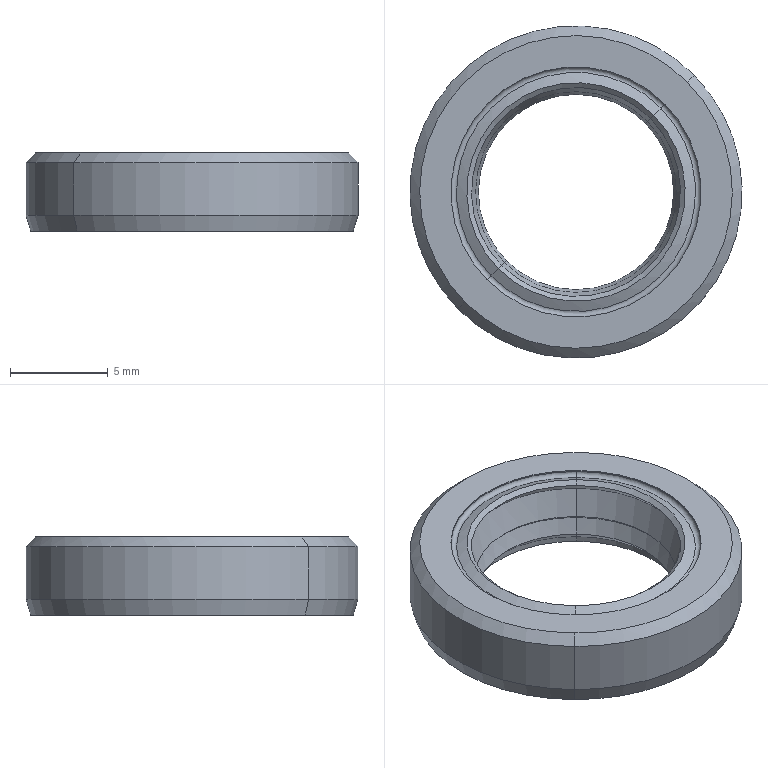Part | SolidWorks | features BaseBody 1 | 1 solid | 53 faces | box 17 x 17 x 4 mm | volume 314.365 mm3 | cone 22 | cylinder 14 | torus 10 | plane 7 | commonest cylinder face diameters 11 x2 12.8 x2 13.5 x2 13.6 x2 15.2 x2 16.2 x2
STEP:
#1=CARTESIAN_POINT('',(387.744,107.08,47.545));
#2=VERTEX_POINT('',#1);
#3=CARTESIAN_POINT('',(387.336,106.678,46.9));
#4=VERTEX_POINT('',#3);
#5=CARTESIAN_POINT('',(387.799,107.135,46.9));
#6=DIRECTION('',(0.7022,-0.712,0.));
#7=DIRECTION('',(0.712,0.7022,0.));
#8=AXIS2_PLACEMENT_3D('',#5,#6,#7);
#9=CIRCLE('',#8,0.65);
#10=EDGE_CURVE('',#2,#4,#9,.T.);
#11=ORIENTED_EDGE('',*,*,#10,.T.);
#12=CARTESIAN_POINT('',(378.864,98.322,46.9));
#13=VERTEX_POINT('',#12);
#14=CARTESIAN_POINT('',(383.1,102.5,46.9));
#15=DIRECTION('',(0.,0.,1.));
#16=DIRECTION('',(0.,-1.,0.));
#17=AXIS2_PLACEMENT_3D('',#14,#15,#16);
#18=CIRCLE('',#17,5.95);
#19=EDGE_CURVE('',#4,#13,#18,.T.);
#20=ORIENTED_EDGE('',*,*,#19,.T.);
#21=CARTESIAN_POINT('',(378.456,97.92,47.545));
#22=VERTEX_POINT('',#21);
#23=CARTESIAN_POINT('',(378.401,97.865,46.9));
#24=DIRECTION('',(-0.7022,0.712,0.));
#25=DIRECTION('',(-0.712,-0.7022,0.));
#26=AXIS2_PLACEMENT_3D('',#23,#24,#25);
#27=CIRCLE('',#26,0.65);
#28=EDGE_CURVE('',#22,#13,#27,.T.);
#29=ORIENTED_EDGE('',*,*,#28,.F.);
#30=CARTESIAN_POINT('',(383.1,102.5,47.545));
#31=DIRECTION('',(0.,0.,1.));
#32=DIRECTION('',(0.712,0.7022,0.));
#33=AXIS2_PLACEMENT_3D('',#30,#31,#32);
#34=CIRCLE('',#33,6.522);
#35=EDGE_CURVE('',#2,#22,#34,.T.);
#36=ORIENTED_EDGE('',*,*,#35,.F.);
#37=EDGE_LOOP('',(#11,#20,#29,#36));
#38=FACE_OUTER_BOUND('',#37,.T.);
#39=CARTESIAN_POINT('',(383.1,102.5,46.9));
#40=DIRECTION('',(0.,0.,1.));
#41=DIRECTION('',(0.712,0.7022,0.));
#42=AXIS2_PLACEMENT_3D('',#39,#40,#41);
#43=TOROIDAL_SURFACE('',#42,6.6,0.65);
#44=ADVANCED_FACE('',(#38),#43,.F.);
#45=ORIENTED_EDGE('',*,*,#28,.T.);
#46=CARTESIAN_POINT('',(383.1,102.5,46.9));
#47=DIRECTION('',(0.,0.,1.));
#48=DIRECTION('',(0.,-1.,0.));
#49=AXIS2_PLACEMENT_3D('',#46,#47,#48);
#50=CIRCLE('',#49,5.95);
#51=EDGE_CURVE('',#13,#4,#50,.T.);
#52=ORIENTED_EDGE('',*,*,#51,.T.);
#53=ORIENTED_EDGE('',*,*,#10,.F.);
#54=CARTESIAN_POINT('',(383.1,102.5,47.545));
#55=DIRECTION('',(0.,0.,1.));
#56=DIRECTION('',(0.712,0.7022,0.));
#57=AXIS2_PLACEMENT_3D('',#54,#55,#56);
#58=CIRCLE('',#57,6.522);
#59=EDGE_CURVE('',#22,#2,#58,.T.);
#60=ORIENTED_EDGE('',*,*,#59,.F.);
#61=EDGE_LOOP('',(#45,#52,#53,#60));
#62=FACE_OUTER_BOUND('',#61,.T.);
#63=CARTESIAN_POINT('',(383.1,102.5,46.9));
#64=DIRECTION('',(0.,0.,1.));
#65=DIRECTION('',(0.712,0.7022,0.));
#66=AXIS2_PLACEMENT_3D('',#63,#64,#65);
#67=TOROIDAL_SURFACE('',#66,6.6,0.65);
#68=ADVANCED_FACE('',(#62),#67,.F.);
#69=CARTESIAN_POINT('',(388.796,108.118,49.5));
#70=VERTEX_POINT('',#69);
#71=CARTESIAN_POINT('',(377.404,96.882,49.5));
#72=VERTEX_POINT('',#71);
#73=CARTESIAN_POINT('',(383.1,102.5,49.5));
#74=DIRECTION('',(0.,0.,1.));
#75=DIRECTION('',(0.712,0.7022,0.));
#76=AXIS2_PLACEMENT_3D('',#73,#74,#75);
#77=CIRCLE('',#76,8.);
#78=EDGE_CURVE('',#70,#72,#77,.T.);
#79=ORIENTED_EDGE('',*,*,#78,.F.);
#80=CARTESIAN_POINT('',(389.152,108.469,49.));
#81=VERTEX_POINT('',#80);
#82=CARTESIAN_POINT('',(388.796,108.118,49.5));
#83=DIRECTION('',(0.5034,0.4965,-0.7071));
#84=VECTOR('',#83,1000.);
#85=LINE('',#82,#84);
#86=EDGE_CURVE('',#70,#81,#85,.T.);
#87=ORIENTED_EDGE('',*,*,#86,.T.);
#88=CARTESIAN_POINT('',(377.048,96.531,49.));
#89=VERTEX_POINT('',#88);
#90=CARTESIAN_POINT('',(383.1,102.5,49.));
#91=DIRECTION('',(0.,0.,-1.));
#92=DIRECTION('',(0.712,0.7022,0.));
#93=AXIS2_PLACEMENT_3D('',#90,#91,#92);
#94=CIRCLE('',#93,8.5);
#95=EDGE_CURVE('',#89,#81,#94,.T.);
#96=ORIENTED_EDGE('',*,*,#95,.F.);
#97=CARTESIAN_POINT('',(377.404,96.882,49.5));
#98=DIRECTION('',(-0.5034,-0.4965,-0.7071));
#99=VECTOR('',#98,1000.);
#100=LINE('',#97,#99);
#101=EDGE_CURVE('',#72,#89,#100,.T.);
#102=ORIENTED_EDGE('',*,*,#101,.F.);
#103=EDGE_LOOP('',(#79,#87,#96,#102));
#104=FACE_OUTER_BOUND('',#103,.T.);
#105=CARTESIAN_POINT('',(383.1,102.5,49.5));
#106=DIRECTION('',(0.,0.,-1.));
#107=DIRECTION('',(-0.712,-0.7022,0.));
#108=AXIS2_PLACEMENT_3D('',#105,#106,#107);
#109=CONICAL_SURFACE('',#108,8.,0.7854);
#110=ADVANCED_FACE('',(#104),#109,.T.);
#111=CARTESIAN_POINT('',(387.079,106.424,49.5));
#112=VERTEX_POINT('',#111);
#113=CARTESIAN_POINT('',(379.121,98.576,49.5));
#114=VERTEX_POINT('',#113);
#115=CARTESIAN_POINT('',(383.1,102.5,49.5));
#116=DIRECTION('',(0.,0.,1.));
#117=DIRECTION('',(0.712,0.7022,0.));
#118=AXIS2_PLACEMENT_3D('',#115,#116,#117);
#119=CIRCLE('',#118,5.588);
#120=EDGE_CURVE('',#112,#114,#119,.T.);
#121=ORIENTED_EDGE('',*,*,#120,.F.);
#122=CARTESIAN_POINT('',(387.454,106.794,49.254));
#123=VERTEX_POINT('',#122);
#124=CARTESIAN_POINT('',(387.079,106.424,49.5));
#125=DIRECTION('',(0.6453,0.6364,-0.4226));
#126=VECTOR('',#125,1000.);
#127=LINE('',#124,#126);
#128=EDGE_CURVE('',#112,#123,#127,.T.);
#129=ORIENTED_EDGE('',*,*,#128,.T.);
#130=CARTESIAN_POINT('',(378.746,98.206,49.254));
#131=VERTEX_POINT('',#130);
#132=CARTESIAN_POINT('',(383.1,102.5,49.254));
#133=DIRECTION('',(0.,0.,1.));
#134=DIRECTION('',(0.712,0.7022,0.));
#135=AXIS2_PLACEMENT_3D('',#132,#133,#134);
#136=CIRCLE('',#135,6.115);
#137=EDGE_CURVE('',#123,#131,#136,.T.);
#138=ORIENTED_EDGE('',*,*,#137,.T.);
#139=CARTESIAN_POINT('',(379.121,98.576,49.5));
#140=DIRECTION('',(-0.6453,-0.6364,-0.4226));
#141=VECTOR('',#140,1000.);
#142=LINE('',#139,#141);
#143=EDGE_CURVE('',#114,#131,#142,.T.);
#144=ORIENTED_EDGE('',*,*,#143,.F.);
#145=EDGE_LOOP('',(#121,#129,#138,#144));
#146=FACE_OUTER_BOUND('',#145,.T.);
#147=CARTESIAN_POINT('',(383.1,102.5,49.5));
#148=DIRECTION('',(0.,0.,-1.));
#149=DIRECTION('',(-0.712,-0.7022,0.));
#150=AXIS2_PLACEMENT_3D('',#147,#148,#149);
#151=CONICAL_SURFACE('',#150,5.588,1.134);
#152=ADVANCED_FACE('',(#146),#151,.T.);
#153=CARTESIAN_POINT('',(379.291,98.743,49.3));
#154=VERTEX_POINT('',#153);
#155=CARTESIAN_POINT('',(386.909,106.257,49.3));
#156=VERTEX_POINT('',#155);
#157=CARTESIAN_POINT('',(383.1,102.5,49.3));
#158=DIRECTION('',(0.,0.,1.));
#159=DIRECTION('',(0.712,0.7022,0.));
#160=AXIS2_PLACEMENT_3D('',#157,#158,#159);
#161=CIRCLE('',#160,5.35);
#162=EDGE_CURVE('',#154,#156,#161,.T.);
#163=ORIENTED_EDGE('',*,*,#162,.F.);
#164=CARTESIAN_POINT('',(379.291,98.743,49.3));
#165=DIRECTION('',(-0.5454,-0.5379,0.6428));
#166=VECTOR('',#165,1000.);
#167=LINE('',#164,#166);
#168=EDGE_CURVE('',#154,#114,#167,.T.);
#169=ORIENTED_EDGE('',*,*,#168,.T.);
#170=CARTESIAN_POINT('',(383.1,102.5,49.5));
#171=DIRECTION('',(0.,0.,1.));
#172=DIRECTION('',(0.712,0.7022,0.));
#173=AXIS2_PLACEMENT_3D('',#170,#171,#172);
#174=CIRCLE('',#173,5.588);
#175=EDGE_CURVE('',#114,#112,#174,.T.);
#176=ORIENTED_EDGE('',*,*,#175,.T.);
#177=CARTESIAN_POINT('',(386.909,106.257,49.3));
#178=DIRECTION('',(0.5454,0.5379,0.6428));
#179=VECTOR('',#178,1000.);
#180=LINE('',#177,#179);
#181=EDGE_CURVE('',#156,#112,#180,.T.);
#182=ORIENTED_EDGE('',*,*,#181,.F.);
#183=EDGE_LOOP('',(#163,#169,#176,#182));
#184=FACE_OUTER_BOUND('',#183,.T.);
#185=CARTESIAN_POINT('',(383.1,102.5,49.3));
#186=DIRECTION('',(0.,0.,1.));
#187=DIRECTION('',(0.712,0.7022,0.));
#188=AXIS2_PLACEMENT_3D('',#185,#186,#187);
#189=CONICAL_SURFACE('',#188,5.35,0.8727);
#190=ADVANCED_FACE('',(#184),#189,.F.);
#191=ORIENTED_EDGE('',*,*,#162,.T.);
#192=CARTESIAN_POINT('',(387.162,106.507,48.876));
#193=VERTEX_POINT('',#192);
#194=CARTESIAN_POINT('',(387.162,106.507,48.876));
#195=DIRECTION('',(0.4576,0.4514,-0.766));
#196=VECTOR('',#195,1000.);
#197=LINE('',#194,#196);
#198=EDGE_CURVE('',#156,#193,#197,.T.);
#199=ORIENTED_EDGE('',*,*,#198,.T.);
#200=CARTESIAN_POINT('',(379.038,98.493,48.876));
#201=VERTEX_POINT('',#200);
#202=CARTESIAN_POINT('',(383.1,102.5,48.876));
#203=DIRECTION('',(0.,0.,1.));
#204=DIRECTION('',(0.712,0.7022,0.));
#205=AXIS2_PLACEMENT_3D('',#202,#203,#204);
#206=CIRCLE('',#205,5.706);
#207=EDGE_CURVE('',#201,#193,#206,.T.);
#208=ORIENTED_EDGE('',*,*,#207,.F.);
#209=CARTESIAN_POINT('',(379.038,98.493,48.876));
#210=DIRECTION('',(-0.4576,-0.4514,-0.766));
#211=VECTOR('',#210,1000.);
#212=LINE('',#209,#211);
#213=EDGE_CURVE('',#154,#201,#212,.T.);
#214=ORIENTED_EDGE('',*,*,#213,.F.);
#215=EDGE_LOOP('',(#191,#199,#208,#214));
#216=FACE_OUTER_BOUND('',#215,.T.);
#217=CARTESIAN_POINT('',(383.1,102.5,48.876));
#218=DIRECTION('',(0.,0.,-1.));
#219=DIRECTION('',(-0.712,-0.7022,0.));
#220=AXIS2_PLACEMENT_3D('',#217,#218,#219);
#221=CONICAL_SURFACE('',#220,5.706,0.6981);
#222=ADVANCED_FACE('',(#216),#221,.F.);
#223=CARTESIAN_POINT('',(379.433,98.884,47.5));
#224=VERTEX_POINT('',#223);
#225=CARTESIAN_POINT('',(386.767,106.116,47.5));
#226=VERTEX_POINT('',#225);
#227=CARTESIAN_POINT('',(383.1,102.5,47.5));
#228=DIRECTION('',(0.,0.,1.));
#229=DIRECTION('',(0.712,0.7022,0.));
#230=AXIS2_PLACEMENT_3D('',#227,#228,#229);
#231=CIRCLE('',#230,5.15);
#232=EDGE_CURVE('',#224,#226,#231,.T.);
#233=ORIENTED_EDGE('',*,*,#232,.F.);
#234=CARTESIAN_POINT('',(379.433,98.884,47.5));
#235=DIRECTION('',(-0.2667,-0.2631,0.9272));
#236=VECTOR('',#235,1000.);
#237=LINE('',#234,#236);
#238=EDGE_CURVE('',#224,#201,#237,.T.);
#239=ORIENTED_EDGE('',*,*,#238,.T.);
#240=ORIENTED_EDGE('',*,*,#207,.T.);
#241=CARTESIAN_POINT('',(386.767,106.116,47.5));
#242=DIRECTION('',(0.2667,0.2631,0.9272));
#243=VECTOR('',#242,1000.);
#244=LINE('',#241,#243);
#245=EDGE_CURVE('',#226,#193,#244,.T.);
#246=ORIENTED_EDGE('',*,*,#245,.F.);
#247=EDGE_LOOP('',(#233,#239,#240,#246));
#248=FACE_OUTER_BOUND('',#247,.T.);
#249=CARTESIAN_POINT('',(383.1,102.5,47.5));
#250=DIRECTION('',(0.,0.,1.));
#251=DIRECTION('',(0.712,0.7022,0.));
#252=AXIS2_PLACEMENT_3D('',#249,#250,#251);
#253=CONICAL_SURFACE('',#252,5.15,0.384);
#254=ADVANCED_FACE('',(#248),#253,.F.);
#255=ORIENTED_EDGE('',*,*,#232,.T.);
#256=CARTESIAN_POINT('',(386.904,106.252,47.307));
#257=VERTEX_POINT('',#256);
#258=CARTESIAN_POINT('',(386.904,106.252,47.307));
#259=DIRECTION('',(0.5034,0.4965,-0.7071));
#260=VECTOR('',#259,1000.);
#261=LINE('',#258,#260);
#262=EDGE_CURVE('',#226,#257,#261,.T.);
#263=ORIENTED_EDGE('',*,*,#262,.T.);
#264=CARTESIAN_POINT('',(379.296,98.748,47.307));
#265=VERTEX_POINT('',#264);
#266=CARTESIAN_POINT('',(383.1,102.5,47.307));
#267=DIRECTION('',(0.,0.,1.));
#268=DIRECTION('',(0.712,0.7022,0.));
#269=AXIS2_PLACEMENT_3D('',#266,#267,#268);
#270=CIRCLE('',#269,5.343);
#271=EDGE_CURVE('',#265,#257,#270,.T.);
#272=ORIENTED_EDGE('',*,*,#271,.F.);
#273=CARTESIAN_POINT('',(379.296,98.748,47.307));
#274=DIRECTION('',(-0.5034,-0.4965,-0.7071));
#275=VECTOR('',#274,1000.);
#276=LINE('',#273,#275);
#277=EDGE_CURVE('',#224,#265,#276,.T.);
#278=ORIENTED_EDGE('',*,*,#277,.F.);
#279=EDGE_LOOP('',(#255,#263,#272,#278));
#280=FACE_OUTER_BOUND('',#279,.T.);
#281=CARTESIAN_POINT('',(383.1,102.5,47.307));
#282=DIRECTION('',(0.,0.,-1.));
#283=DIRECTION('',(-0.712,-0.7022,0.));
#284=AXIS2_PLACEMENT_3D('',#281,#282,#283);
#285=CONICAL_SURFACE('',#284,5.343,0.7854);
#286=ADVANCED_FACE('',(#280),#285,.F.);
#287=CARTESIAN_POINT('',(379.54,98.989,46.5));
#288=VERTEX_POINT('',#287);
#289=CARTESIAN_POINT('',(386.66,106.011,46.5));
#290=VERTEX_POINT('',#289);
#291=CARTESIAN_POINT('',(383.1,102.5,46.5));
#292=DIRECTION('',(0.,0.,1.));
#293=DIRECTION('',(0.712,0.7022,0.));
#294=AXIS2_PLACEMENT_3D('',#291,#292,#293);
#295=CIRCLE('',#294,5.);
#296=EDGE_CURVE('',#288,#290,#295,.T.);
#297=ORIENTED_EDGE('',*,*,#296,.F.);
#298=CARTESIAN_POINT('',(379.54,98.989,46.5));
#299=DIRECTION('',(-0.2782,-0.2744,0.9205));
#300=VECTOR('',#299,1000.);
#301=LINE('',#298,#300);
#302=EDGE_CURVE('',#288,#265,#301,.T.);
#303=ORIENTED_EDGE('',*,*,#302,.T.);
#304=ORIENTED_EDGE('',*,*,#271,.T.);
#305=CARTESIAN_POINT('',(386.66,106.011,46.5));
#306=DIRECTION('',(0.2782,0.2744,0.9205));
#307=VECTOR('',#306,1000.);
#308=LINE('',#305,#307);
#309=EDGE_CURVE('',#290,#257,#308,.T.);
#310=ORIENTED_EDGE('',*,*,#309,.F.);
#311=EDGE_LOOP('',(#297,#303,#304,#310));
#312=FACE_OUTER_BOUND('',#311,.T.);
#313=CARTESIAN_POINT('',(383.1,102.5,46.5));
#314=DIRECTION('',(0.,0.,1.));
#315=DIRECTION('',(0.712,0.7022,0.));
#316=AXIS2_PLACEMENT_3D('',#313,#314,#315);
#317=CONICAL_SURFACE('',#316,5.,0.4014);
#318=ADVANCED_FACE('',(#312),#317,.F.);
#319=ORIENTED_EDGE('',*,*,#296,.T.);
#320=CARTESIAN_POINT('',(387.016,106.362,46.));
#321=VERTEX_POINT('',#320);
#322=CARTESIAN_POINT('',(387.016,106.362,46.));
#323=DIRECTION('',(0.5034,0.4965,-0.7071));
#324=VECTOR('',#323,1000.);
#325=LINE('',#322,#324);
#326=EDGE_CURVE('',#290,#321,#325,.T.);
#327=ORIENTED_EDGE('',*,*,#326,.T.);
#328=CARTESIAN_POINT('',(379.184,98.638,46.));
#329=VERTEX_POINT('',#328);
#330=CARTESIAN_POINT('',(383.1,102.5,46.));
#331=DIRECTION('',(0.,0.,1.));
#332=DIRECTION('',(0.712,0.7022,0.));
#333=AXIS2_PLACEMENT_3D('',#330,#331,#332);
#334=CIRCLE('',#333,5.5);
#335=EDGE_CURVE('',#329,#321,#334,.T.);
#336=ORIENTED_EDGE('',*,*,#335,.F.);
#337=CARTESIAN_POINT('',(379.184,98.638,46.));
#338=DIRECTION('',(-0.5034,-0.4965,-0.7071));
#339=VECTOR('',#338,1000.);
#340=LINE('',#337,#339);
#341=EDGE_CURVE('',#288,#329,#340,.T.);
#342=ORIENTED_EDGE('',*,*,#341,.F.);
#343=EDGE_LOOP('',(#319,#327,#336,#342));
#344=FACE_OUTER_BOUND('',#343,.T.);
#345=CARTESIAN_POINT('',(383.1,102.5,46.));
#346=DIRECTION('',(0.,0.,-1.));
#347=DIRECTION('',(-0.712,-0.7022,0.));
#348=AXIS2_PLACEMENT_3D('',#345,#346,#347);
#349=CONICAL_SURFACE('',#348,5.5,0.7854);
#350=ADVANCED_FACE('',(#344),#349,.F.);
#351=CARTESIAN_POINT('',(379.184,98.638,45.7));
#352=VERTEX_POINT('',#351);
#353=CARTESIAN_POINT('',(387.016,106.362,45.7));
#354=VERTEX_POINT('',#353);
#355=CARTESIAN_POINT('',(383.1,102.5,45.7));
#356=DIRECTION('',(0.,0.,1.));
#357=DIRECTION('',(0.712,0.7022,0.));
#358=AXIS2_PLACEMENT_3D('',#355,#356,#357);
#359=CIRCLE('',#358,5.5);
#360=EDGE_CURVE('',#352,#354,#359,.T.);
#361=ORIENTED_EDGE('',*,*,#360,.F.);
#362=CARTESIAN_POINT('',(379.184,98.638,49.5));
#363=DIRECTION('',(0.,0.,1.));
#364=VECTOR('',#363,1000.);
#365=LINE('',#362,#364);
#366=EDGE_CURVE('',#352,#329,#365,.T.);
#367=ORIENTED_EDGE('',*,*,#366,.T.);
#368=ORIENTED_EDGE('',*,*,#335,.T.);
#369=CARTESIAN_POINT('',(387.016,106.362,49.5));
#370=DIRECTION('',(0.,0.,1.));
#371=VECTOR('',#370,1000.);
#372=LINE('',#369,#371);
#373=EDGE_CURVE('',#354,#321,#372,.T.);
#374=ORIENTED_EDGE('',*,*,#373,.F.);
#375=EDGE_LOOP('',(#361,#367,#368,#374));
#376=FACE_OUTER_BOUND('',#375,.T.);
#377=CARTESIAN_POINT('',(383.1,102.5,49.5));
#378=DIRECTION('',(0.,0.,1.));
#379=DIRECTION('',(0.712,0.7022,0.));
#380=AXIS2_PLACEMENT_3D('',#377,#378,#379);
#381=CYLINDRICAL_SURFACE('',#380,5.5);
#382=ADVANCED_FACE('',(#376),#381,.F.);
#383=CARTESIAN_POINT('',(387.906,107.24,45.7));
#384=VERTEX_POINT('',#383);
#385=CARTESIAN_POINT('',(378.294,97.76,45.7));
#386=VERTEX_POINT('',#385);
#387=CARTESIAN_POINT('',(383.1,102.5,45.7));
#388=DIRECTION('',(0.,0.,1.));
#389=DIRECTION('',(0.712,0.7022,0.));
#390=AXIS2_PLACEMENT_3D('',#387,#388,#389);
#391=CIRCLE('',#390,6.75);
#392=EDGE_CURVE('',#384,#386,#391,.T.);
#393=ORIENTED_EDGE('',*,*,#392,.T.);
#394=CARTESIAN_POINT('',(378.294,97.76,46.268));
#395=VERTEX_POINT('',#394);
#396=CARTESIAN_POINT('',(378.294,97.76,49.5));
#397=DIRECTION('',(0.,0.,1.));
#398=VECTOR('',#397,1000.);
#399=LINE('',#396,#398);
#400=EDGE_CURVE('',#386,#395,#399,.T.);
#401=ORIENTED_EDGE('',*,*,#400,.T.);
#402=CARTESIAN_POINT('',(387.906,107.24,46.268));
#403=VERTEX_POINT('',#402);
#404=CARTESIAN_POINT('',(383.1,102.5,46.268));
#405=DIRECTION('',(0.,0.,1.));
#406=DIRECTION('',(0.712,0.7022,0.));
#407=AXIS2_PLACEMENT_3D('',#404,#405,#406);
#408=CIRCLE('',#407,6.75);
#409=EDGE_CURVE('',#403,#395,#408,.T.);
#410=ORIENTED_EDGE('',*,*,#409,.F.);
#411=CARTESIAN_POINT('',(387.906,107.24,49.5));
#412=DIRECTION('',(0.,0.,1.));
#413=VECTOR('',#412,1000.);
#414=LINE('',#411,#413);
#415=EDGE_CURVE('',#384,#403,#414,.T.);
#416=ORIENTED_EDGE('',*,*,#415,.F.);
#417=EDGE_LOOP('',(#393,#401,#410,#416));
#418=FACE_OUTER_BOUND('',#417,.T.);
#419=CARTESIAN_POINT('',(383.1,102.5,49.5));
#420=DIRECTION('',(0.,0.,1.));
#421=DIRECTION('',(0.712,0.7022,0.));
#422=AXIS2_PLACEMENT_3D('',#419,#420,#421);
#423=CYLINDRICAL_SURFACE('',#422,6.75);
#424=ADVANCED_FACE('',(#418),#423,.T.);
#425=ORIENTED_EDGE('',*,*,#51,.F.);
#426=CARTESIAN_POINT('',(378.401,97.865,46.9));
#427=DIRECTION('',(-0.7022,0.712,0.));
#428=DIRECTION('',(-0.712,-0.7022,0.));
#429=AXIS2_PLACEMENT_3D('',#426,#427,#428);
#430=CIRCLE('',#429,0.65);
#431=EDGE_CURVE('',#13,#395,#430,.T.);
#432=ORIENTED_EDGE('',*,*,#431,.T.);
#433=CARTESIAN_POINT('',(383.1,102.5,46.268));
#434=DIRECTION('',(0.,0.,1.));
#435=DIRECTION('',(0.712,0.7022,0.));
#436=AXIS2_PLACEMENT_3D('',#433,#434,#435);
#437=CIRCLE('',#436,6.75);
#438=EDGE_CURVE('',#395,#403,#437,.T.);
#439=ORIENTED_EDGE('',*,*,#438,.T.);
#440=CARTESIAN_POINT('',(387.799,107.135,46.9));
#441=DIRECTION('',(0.7022,-0.712,0.));
#442=DIRECTION('',(0.712,0.7022,0.));
#443=AXIS2_PLACEMENT_3D('',#440,#441,#442);
#444=CIRCLE('',#443,0.65);
#445=EDGE_CURVE('',#4,#403,#444,.T.);
#446=ORIENTED_EDGE('',*,*,#445,.F.);
#447=EDGE_LOOP('',(#425,#432,#439,#446));
#448=FACE_OUTER_BOUND('',#447,.T.);
#449=CARTESIAN_POINT('',(383.1,102.5,46.9));
#450=DIRECTION('',(0.,0.,1.));
#451=DIRECTION('',(0.712,0.7022,0.));
#452=AXIS2_PLACEMENT_3D('',#449,#450,#451);
#453=TOROIDAL_SURFACE('',#452,6.6,0.65);
#454=ADVANCED_FACE('',(#448),#453,.F.);
#455=ORIENTED_EDGE('',*,*,#35,.T.);
#456=CARTESIAN_POINT('',(378.259,97.725,48.4));
#457=VERTEX_POINT('',#456);
#458=CARTESIAN_POINT('',(378.259,97.725,48.4));
#459=DIRECTION('',(-0.22,-0.217,0.9511));
#460=VECTOR('',#459,1000.);
#461=LINE('',#458,#460);
#462=EDGE_CURVE('',#22,#457,#461,.T.);
#463=ORIENTED_EDGE('',*,*,#462,.T.);
#464=CARTESIAN_POINT('',(387.941,107.275,48.4));
#465=VERTEX_POINT('',#464);
#466=CARTESIAN_POINT('',(383.1,102.5,48.4));
#467=DIRECTION('',(0.,0.,1.));
#468=DIRECTION('',(0.712,0.7022,0.));
#469=AXIS2_PLACEMENT_3D('',#466,#467,#468);
#470=CIRCLE('',#469,6.8);
#471=EDGE_CURVE('',#465,#457,#470,.T.);
#472=ORIENTED_EDGE('',*,*,#471,.F.);
#473=CARTESIAN_POINT('',(387.941,107.275,48.4));
#474=DIRECTION('',(0.22,0.217,0.9511));
#475=VECTOR('',#474,1000.);
#476=LINE('',#473,#475);
#477=EDGE_CURVE('',#2,#465,#476,.T.);
#478=ORIENTED_EDGE('',*,*,#477,.F.);
#479=EDGE_LOOP('',(#455,#463,#472,#478));
#480=FACE_OUTER_BOUND('',#479,.T.);
#481=CARTESIAN_POINT('',(383.1,102.5,48.4));
#482=DIRECTION('',(0.,0.,1.));
#483=DIRECTION('',(0.712,0.7022,0.));
#484=AXIS2_PLACEMENT_3D('',#481,#482,#483);
#485=CONICAL_SURFACE('',#484,6.8,0.3142);
#486=ADVANCED_FACE('',(#480),#485,.T.);
#487=CARTESIAN_POINT('',(377.868,97.34,48.4));
#488=VERTEX_POINT('',#487);
#489=CARTESIAN_POINT('',(388.332,107.66,48.4));
#490=VERTEX_POINT('',#489);
#491=CARTESIAN_POINT('',(383.1,102.5,48.4));
#492=DIRECTION('',(0.,0.,1.));
#493=DIRECTION('',(0.712,0.7022,0.));
#494=AXIS2_PLACEMENT_3D('',#491,#492,#493);
#495=CIRCLE('',#494,7.348);
#496=EDGE_CURVE('',#488,#490,#495,.T.);
#497=ORIENTED_EDGE('',*,*,#496,.T.);
#498=CARTESIAN_POINT('',(388.44,107.767,45.5));
#499=VERTEX_POINT('',#498);
#500=CARTESIAN_POINT('',(388.44,107.767,45.5));
#501=DIRECTION('',(0.03726,0.03675,-0.9986));
#502=VECTOR('',#501,1000.);
#503=LINE('',#500,#502);
#504=EDGE_CURVE('',#490,#499,#503,.T.);
#505=ORIENTED_EDGE('',*,*,#504,.T.);
#506=CARTESIAN_POINT('',(377.76,97.233,45.5));
#507=VERTEX_POINT('',#506);
#508=CARTESIAN_POINT('',(383.1,102.5,45.5));
#509=DIRECTION('',(0.,0.,1.));
#510=DIRECTION('',(0.712,0.7022,0.));
#511=AXIS2_PLACEMENT_3D('',#508,#509,#510);
#512=CIRCLE('',#511,7.5);
#513=EDGE_CURVE('',#507,#499,#512,.T.);
#514=ORIENTED_EDGE('',*,*,#513,.F.);
#515=CARTESIAN_POINT('',(377.76,97.233,45.5));
#516=DIRECTION('',(-0.03726,-0.03675,-0.9986));
#517=VECTOR('',#516,1000.);
#518=LINE('',#515,#517);
#519=EDGE_CURVE('',#488,#507,#518,.T.);
#520=ORIENTED_EDGE('',*,*,#519,.F.);
#521=EDGE_LOOP('',(#497,#505,#514,#520));
#522=FACE_OUTER_BOUND('',#521,.T.);
#523=CARTESIAN_POINT('',(383.1,102.5,45.5));
#524=DIRECTION('',(0.,0.,-1.));
#525=DIRECTION('',(-0.712,-0.7022,0.));
#526=AXIS2_PLACEMENT_3D('',#523,#524,#525);
#527=CONICAL_SURFACE('',#526,7.5,0.05236);
#528=ADVANCED_FACE('',(#522),#527,.F.);
#529=CARTESIAN_POINT('',(388.978,108.297,45.5));
#530=VERTEX_POINT('',#529);
#531=CARTESIAN_POINT('',(377.222,96.703,45.5));
#532=VERTEX_POINT('',#531);
#533=CARTESIAN_POINT('',(383.1,102.5,45.5));
#534=DIRECTION('',(0.,0.,1.));
#535=DIRECTION('',(0.712,0.7022,0.));
#536=AXIS2_PLACEMENT_3D('',#533,#534,#535);
#537=CIRCLE('',#536,8.255);
#538=EDGE_CURVE('',#530,#532,#537,.T.);
#539=ORIENTED_EDGE('',*,*,#538,.T.);
#540=CARTESIAN_POINT('',(377.048,96.531,46.3));
#541=VERTEX_POINT('',#540);
#542=CARTESIAN_POINT('',(377.048,96.531,46.3));
#543=DIRECTION('',(-0.2082,-0.2053,0.9563));
#544=VECTOR('',#543,1000.);
#545=LINE('',#542,#544);
#546=EDGE_CURVE('',#532,#541,#545,.T.);
#547=ORIENTED_EDGE('',*,*,#546,.T.);
#548=CARTESIAN_POINT('',(389.152,108.469,46.3));
#549=VERTEX_POINT('',#548);
#550=CARTESIAN_POINT('',(383.1,102.5,46.3));
#551=DIRECTION('',(0.,0.,1.));
#552=DIRECTION('',(0.712,0.7022,0.));
#553=AXIS2_PLACEMENT_3D('',#550,#551,#552);
#554=CIRCLE('',#553,8.5);
#555=EDGE_CURVE('',#549,#541,#554,.T.);
#556=ORIENTED_EDGE('',*,*,#555,.F.);
#557=CARTESIAN_POINT('',(389.152,108.469,46.3));
#558=DIRECTION('',(0.2082,0.2053,0.9563));
#559=VECTOR('',#558,1000.);
#560=LINE('',#557,#559);
#561=EDGE_CURVE('',#530,#549,#560,.T.);
#562=ORIENTED_EDGE('',*,*,#561,.F.);
#563=EDGE_LOOP('',(#539,#547,#556,#562));
#564=FACE_OUTER_BOUND('',#563,.T.);
#565=CARTESIAN_POINT('',(383.1,102.5,46.3));
#566=DIRECTION('',(0.,0.,1.));
#567=DIRECTION('',(0.712,0.7022,0.));
#568=AXIS2_PLACEMENT_3D('',#565,#566,#567);
#569=CONICAL_SURFACE('',#568,8.5,0.2967);
#570=ADVANCED_FACE('',(#564),#569,.T.);
#571=ORIENTED_EDGE('',*,*,#555,.T.);
#572=CARTESIAN_POINT('',(377.048,96.531,49.5));
#573=DIRECTION('',(0.,0.,1.));
#574=VECTOR('',#573,1000.);
#575=LINE('',#572,#574);
#576=EDGE_CURVE('',#541,#89,#575,.T.);
#577=ORIENTED_EDGE('',*,*,#576,.T.);
#578=ORIENTED_EDGE('',*,*,#95,.T.);
#579=CARTESIAN_POINT('',(389.152,108.469,49.5));
#580=DIRECTION('',(0.,0.,1.));
#581=VECTOR('',#580,1000.);
#582=LINE('',#579,#581);
#583=EDGE_CURVE('',#549,#81,#582,.T.);
#584=ORIENTED_EDGE('',*,*,#583,.F.);
#585=EDGE_LOOP('',(#571,#577,#578,#584));
#586=FACE_OUTER_BOUND('',#585,.T.);
#587=CARTESIAN_POINT('',(383.1,102.5,49.5));
#588=DIRECTION('',(0.,0.,1.));
#589=DIRECTION('',(0.712,0.7022,0.));
#590=AXIS2_PLACEMENT_3D('',#587,#588,#589);
#591=CYLINDRICAL_SURFACE('',#590,8.5);
#592=ADVANCED_FACE('',(#586),#591,.T.);
#593=CARTESIAN_POINT('',(378.543,98.006,49.435));
#594=VERTEX_POINT('',#593);
#595=CARTESIAN_POINT('',(387.657,106.994,49.435));
#596=VERTEX_POINT('',#595);
#597=CARTESIAN_POINT('',(383.1,102.5,49.435));
#598=DIRECTION('',(0.,0.,1.));
#599=DIRECTION('',(0.712,0.7022,0.));
#600=AXIS2_PLACEMENT_3D('',#597,#598,#599);
#601=CIRCLE('',#600,6.4);
#602=EDGE_CURVE('',#594,#596,#601,.T.);
#603=ORIENTED_EDGE('',*,*,#602,.F.);
#604=CARTESIAN_POINT('',(378.543,98.006,49.5));
#605=VERTEX_POINT('',#604);
#606=CARTESIAN_POINT('',(378.543,98.006,49.5));
#607=DIRECTION('',(0.,0.,1.));
#608=VECTOR('',#607,1000.);
#609=LINE('',#606,#608);
#610=EDGE_CURVE('',#594,#605,#609,.T.);
#611=ORIENTED_EDGE('',*,*,#610,.T.);
#612=CARTESIAN_POINT('',(387.657,106.994,49.5));
#613=VERTEX_POINT('',#612);
#614=CARTESIAN_POINT('',(383.1,102.5,49.5));
#615=DIRECTION('',(0.,0.,1.));
#616=DIRECTION('',(0.712,0.7022,0.));
#617=AXIS2_PLACEMENT_3D('',#614,#615,#616);
#618=CIRCLE('',#617,6.4);
#619=EDGE_CURVE('',#605,#613,#618,.T.);
#620=ORIENTED_EDGE('',*,*,#619,.T.);
#621=CARTESIAN_POINT('',(387.657,106.994,49.5));
#622=DIRECTION('',(0.,0.,1.));
#623=VECTOR('',#622,1000.);
#624=LINE('',#621,#623);
#625=EDGE_CURVE('',#596,#613,#624,.T.);
#626=ORIENTED_EDGE('',*,*,#625,.F.);
#627=EDGE_LOOP('',(#603,#611,#620,#626));
#628=FACE_OUTER_BOUND('',#627,.T.);
#629=CARTESIAN_POINT('',(383.1,102.5,49.5));
#630=DIRECTION('',(0.,0.,1.));
#631=DIRECTION('',(0.712,0.7022,0.));
#632=AXIS2_PLACEMENT_3D('',#629,#630,#631);
#633=CYLINDRICAL_SURFACE('',#632,6.4);
#634=ADVANCED_FACE('',(#628),#633,.F.);
#635=CARTESIAN_POINT('',(383.1,102.5,49.254));
#636=DIRECTION('',(0.,0.,1.));
#637=DIRECTION('',(0.712,0.7022,0.));
#638=AXIS2_PLACEMENT_3D('',#635,#636,#637);
#639=CIRCLE('',#638,6.115);
#640=EDGE_CURVE('',#131,#123,#639,.T.);
#641=ORIENTED_EDGE('',*,*,#640,.F.);
#642=CARTESIAN_POINT('',(378.686,98.146,49.435));
#643=DIRECTION('',(-0.7022,0.712,0.));
#644=DIRECTION('',(-0.712,-0.7022,0.));
#645=AXIS2_PLACEMENT_3D('',#642,#643,#644);
#646=CIRCLE('',#645,0.2);
#647=EDGE_CURVE('',#131,#594,#646,.T.);
#648=ORIENTED_EDGE('',*,*,#647,.T.);
#649=ORIENTED_EDGE('',*,*,#602,.T.);
#650=CARTESIAN_POINT('',(387.514,106.854,49.435));
#651=DIRECTION('',(0.7022,-0.712,0.));
#652=DIRECTION('',(0.712,0.7022,0.));
#653=AXIS2_PLACEMENT_3D('',#650,#651,#652);
#654=CIRCLE('',#653,0.2);
#655=EDGE_CURVE('',#123,#596,#654,.T.);
#656=ORIENTED_EDGE('',*,*,#655,.F.);
#657=EDGE_LOOP('',(#641,#648,#649,#656));
#658=FACE_OUTER_BOUND('',#657,.T.);
#659=CARTESIAN_POINT('',(383.1,102.5,49.435));
#660=DIRECTION('',(0.,0.,1.));
#661=DIRECTION('',(0.712,0.7022,0.));
#662=AXIS2_PLACEMENT_3D('',#659,#660,#661);
#663=TOROIDAL_SURFACE('',#662,6.2,0.2);
#664=ADVANCED_FACE('',(#658),#663,.F.);
#665=ORIENTED_EDGE('',*,*,#647,.F.);
#666=ORIENTED_EDGE('',*,*,#137,.F.);
#667=ORIENTED_EDGE('',*,*,#655,.T.);
#668=CARTESIAN_POINT('',(383.1,102.5,49.435));
#669=DIRECTION('',(0.,0.,1.));
#670=DIRECTION('',(0.712,0.7022,0.));
#671=AXIS2_PLACEMENT_3D('',#668,#669,#670);
#672=CIRCLE('',#671,6.4);
#673=EDGE_CURVE('',#596,#594,#672,.T.);
#674=ORIENTED_EDGE('',*,*,#673,.T.);
#675=EDGE_LOOP('',(#665,#666,#667,#674));
#676=FACE_OUTER_BOUND('',#675,.T.);
#677=CARTESIAN_POINT('',(383.1,102.5,49.435));
#678=DIRECTION('',(0.,0.,1.));
#679=DIRECTION('',(0.712,0.7022,0.));
#680=AXIS2_PLACEMENT_3D('',#677,#678,#679);
#681=TOROIDAL_SURFACE('',#680,6.2,0.2);
#682=ADVANCED_FACE('',(#676),#681,.F.);
#683=ORIENTED_EDGE('',*,*,#610,.F.);
#684=ORIENTED_EDGE('',*,*,#673,.F.);
#685=ORIENTED_EDGE('',*,*,#625,.T.);
#686=CARTESIAN_POINT('',(383.1,102.5,49.5));
#687=DIRECTION('',(0.,0.,1.));
#688=DIRECTION('',(0.712,0.7022,0.));
#689=AXIS2_PLACEMENT_3D('',#686,#687,#688);
#690=CIRCLE('',#689,6.4);
#691=EDGE_CURVE('',#613,#605,#690,.T.);
#692=ORIENTED_EDGE('',*,*,#691,.T.);
#693=EDGE_LOOP('',(#683,#684,#685,#692));
#694=FACE_OUTER_BOUND('',#693,.T.);
#695=CARTESIAN_POINT('',(383.1,102.5,49.5));
#696=DIRECTION('',(0.,0.,1.));
#697=DIRECTION('',(0.712,0.7022,0.));
#698=AXIS2_PLACEMENT_3D('',#695,#696,#697);
#699=CYLINDRICAL_SURFACE('',#698,6.4);
#700=ADVANCED_FACE('',(#694),#699,.F.);
#701=CARTESIAN_POINT('',(383.1,102.5,49.5));
#702=DIRECTION('',(0.,0.,1.));
#703=DIRECTION('',(0.712,0.7022,0.));
#704=AXIS2_PLACEMENT_3D('',#701,#702,#703);
#705=CIRCLE('',#704,8.);
#706=EDGE_CURVE('',#72,#70,#705,.T.);
#707=ORIENTED_EDGE('',*,*,#706,.T.);
#708=ORIENTED_EDGE('',*,*,#78,.T.);
#709=EDGE_LOOP('',(#707,#708));
#710=FACE_OUTER_BOUND('',#709,.T.);
#711=ORIENTED_EDGE('',*,*,#691,.F.);
#712=ORIENTED_EDGE('',*,*,#619,.F.);
#713=EDGE_LOOP('',(#711,#712));
#714=FACE_BOUND('',#713,.T.);
#715=CARTESIAN_POINT('',(378.2,107.468,49.5));
#716=DIRECTION('',(0.,0.,1.));
#717=DIRECTION('',(0.712,0.7022,0.));
#718=AXIS2_PLACEMENT_3D('',#715,#716,#717);
#719=PLANE('',#718);
#720=ADVANCED_FACE('',(#710,#714),#719,.T.);
#721=ORIENTED_EDGE('',*,*,#576,.F.);
#722=CARTESIAN_POINT('',(383.1,102.5,46.3));
#723=DIRECTION('',(0.,0.,1.));
#724=DIRECTION('',(0.712,0.7022,0.));
#725=AXIS2_PLACEMENT_3D('',#722,#723,#724);
#726=CIRCLE('',#725,8.5);
#727=EDGE_CURVE('',#541,#549,#726,.T.);
#728=ORIENTED_EDGE('',*,*,#727,.T.);
#729=ORIENTED_EDGE('',*,*,#583,.T.);
#730=CARTESIAN_POINT('',(383.1,102.5,49.));
#731=DIRECTION('',(0.,0.,-1.));
#732=DIRECTION('',(0.712,0.7022,0.));
#733=AXIS2_PLACEMENT_3D('',#730,#731,#732);
#734=CIRCLE('',#733,8.5);
#735=EDGE_CURVE('',#81,#89,#734,.T.);
#736=ORIENTED_EDGE('',*,*,#735,.T.);
#737=EDGE_LOOP('',(#721,#728,#729,#736));
#738=FACE_OUTER_BOUND('',#737,.T.);
#739=CARTESIAN_POINT('',(383.1,102.5,49.5));
#740=DIRECTION('',(0.,0.,1.));
#741=DIRECTION('',(0.712,0.7022,0.));
#742=AXIS2_PLACEMENT_3D('',#739,#740,#741);
#743=CYLINDRICAL_SURFACE('',#742,8.5);
#744=ADVANCED_FACE('',(#738),#743,.T.);
#745=ORIENTED_EDGE('',*,*,#546,.F.);
#746=CARTESIAN_POINT('',(383.1,102.5,45.5));
#747=DIRECTION('',(0.,0.,1.));
#748=DIRECTION('',(0.712,0.7022,0.));
#749=AXIS2_PLACEMENT_3D('',#746,#747,#748);
#750=CIRCLE('',#749,8.255);
#751=EDGE_CURVE('',#532,#530,#750,.T.);
#752=ORIENTED_EDGE('',*,*,#751,.T.);
#753=ORIENTED_EDGE('',*,*,#561,.T.);
#754=ORIENTED_EDGE('',*,*,#727,.F.);
#755=EDGE_LOOP('',(#745,#752,#753,#754));
#756=FACE_OUTER_BOUND('',#755,.T.);
#757=CARTESIAN_POINT('',(383.1,102.5,46.3));
#758=DIRECTION('',(0.,0.,1.));
#759=DIRECTION('',(0.712,0.7022,0.));
#760=AXIS2_PLACEMENT_3D('',#757,#758,#759);
#761=CONICAL_SURFACE('',#760,8.5,0.2967);
#762=ADVANCED_FACE('',(#756),#761,.T.);
#763=ORIENTED_EDGE('',*,*,#513,.T.);
#764=CARTESIAN_POINT('',(383.1,102.5,45.5));
#765=DIRECTION('',(0.,0.,1.));
#766=DIRECTION('',(0.712,0.7022,0.));
#767=AXIS2_PLACEMENT_3D('',#764,#765,#766);
#768=CIRCLE('',#767,7.5);
#769=EDGE_CURVE('',#499,#507,#768,.T.);
#770=ORIENTED_EDGE('',*,*,#769,.T.);
#771=EDGE_LOOP('',(#763,#770));
#772=FACE_BOUND('',#771,.T.);
#773=ORIENTED_EDGE('',*,*,#538,.F.);
#774=ORIENTED_EDGE('',*,*,#751,.F.);
#775=EDGE_LOOP('',(#773,#774));
#776=FACE_OUTER_BOUND('',#775,.T.);
#777=CARTESIAN_POINT('',(378.2,107.468,45.5));
#778=DIRECTION('',(0.,0.,-1.));
#779=DIRECTION('',(-0.712,-0.7022,0.));
#780=AXIS2_PLACEMENT_3D('',#777,#778,#779);
#781=PLANE('',#780);
#782=ADVANCED_FACE('',(#772,#776),#781,.T.);
#783=ORIENTED_EDGE('',*,*,#504,.F.);
#784=CARTESIAN_POINT('',(383.1,102.5,48.4));
#785=DIRECTION('',(0.,0.,1.));
#786=DIRECTION('',(0.712,0.7022,0.));
#787=AXIS2_PLACEMENT_3D('',#784,#785,#786);
#788=CIRCLE('',#787,7.348);
#789=EDGE_CURVE('',#490,#488,#788,.T.);
#790=ORIENTED_EDGE('',*,*,#789,.T.);
#791=ORIENTED_EDGE('',*,*,#519,.T.);
#792=ORIENTED_EDGE('',*,*,#769,.F.);
#793=EDGE_LOOP('',(#783,#790,#791,#792));
#794=FACE_OUTER_BOUND('',#793,.T.);
#795=CARTESIAN_POINT('',(383.1,102.5,45.5));
#796=DIRECTION('',(0.,0.,-1.));
#797=DIRECTION('',(-0.712,-0.7022,0.));
#798=AXIS2_PLACEMENT_3D('',#795,#796,#797);
#799=CONICAL_SURFACE('',#798,7.5,0.05236);
#800=ADVANCED_FACE('',(#794),#799,.F.);
#801=ORIENTED_EDGE('',*,*,#471,.T.);
#802=CARTESIAN_POINT('',(383.1,102.5,48.4));
#803=DIRECTION('',(0.,0.,1.));
#804=DIRECTION('',(0.712,0.7022,0.));
#805=AXIS2_PLACEMENT_3D('',#802,#803,#804);
#806=CIRCLE('',#805,6.8);
#807=EDGE_CURVE('',#457,#465,#806,.T.);
#808=ORIENTED_EDGE('',*,*,#807,.T.);
#809=EDGE_LOOP('',(#801,#808));
#810=FACE_BOUND('',#809,.T.);
#811=ORIENTED_EDGE('',*,*,#496,.F.);
#812=ORIENTED_EDGE('',*,*,#789,.F.);
#813=EDGE_LOOP('',(#811,#812));
#814=FACE_OUTER_BOUND('',#813,.T.);
#815=CARTESIAN_POINT('',(378.2,107.468,48.4));
#816=DIRECTION('',(0.,0.,-1.));
#817=DIRECTION('',(-0.712,-0.7022,0.));
#818=AXIS2_PLACEMENT_3D('',#815,#816,#817);
#819=PLANE('',#818);
#820=ADVANCED_FACE('',(#810,#814),#819,.T.);
#821=ORIENTED_EDGE('',*,*,#462,.F.);
#822=ORIENTED_EDGE('',*,*,#59,.T.);
#823=ORIENTED_EDGE('',*,*,#477,.T.);
#824=ORIENTED_EDGE('',*,*,#807,.F.);
#825=EDGE_LOOP('',(#821,#822,#823,#824));
#826=FACE_OUTER_BOUND('',#825,.T.);
#827=CARTESIAN_POINT('',(383.1,102.5,48.4));
#828=DIRECTION('',(0.,0.,1.));
#829=DIRECTION('',(0.712,0.7022,0.));
#830=AXIS2_PLACEMENT_3D('',#827,#828,#829);
#831=CONICAL_SURFACE('',#830,6.8,0.3142);
#832=ADVANCED_FACE('',(#826),#831,.T.);
#833=ORIENTED_EDGE('',*,*,#19,.F.);
#834=ORIENTED_EDGE('',*,*,#445,.T.);
#835=ORIENTED_EDGE('',*,*,#409,.T.);
#836=ORIENTED_EDGE('',*,*,#431,.F.);
#837=EDGE_LOOP('',(#833,#834,#835,#836));
#838=FACE_OUTER_BOUND('',#837,.T.);
#839=CARTESIAN_POINT('',(383.1,102.5,46.9));
#840=DIRECTION('',(0.,0.,1.));
#841=DIRECTION('',(0.712,0.7022,0.));
#842=AXIS2_PLACEMENT_3D('',#839,#840,#841);
#843=TOROIDAL_SURFACE('',#842,6.6,0.65);
#844=ADVANCED_FACE('',(#838),#843,.F.);
#845=ORIENTED_EDGE('',*,*,#400,.F.);
#846=CARTESIAN_POINT('',(383.1,102.5,45.7));
#847=DIRECTION('',(0.,0.,1.));
#848=DIRECTION('',(0.712,0.7022,0.));
#849=AXIS2_PLACEMENT_3D('',#846,#847,#848);
#850=CIRCLE('',#849,6.75);
#851=EDGE_CURVE('',#386,#384,#850,.T.);
#852=ORIENTED_EDGE('',*,*,#851,.T.);
#853=ORIENTED_EDGE('',*,*,#415,.T.);
#854=ORIENTED_EDGE('',*,*,#438,.F.);
#855=EDGE_LOOP('',(#845,#852,#853,#854));
#856=FACE_OUTER_BOUND('',#855,.T.);
#857=CARTESIAN_POINT('',(383.1,102.5,49.5));
#858=DIRECTION('',(0.,0.,1.));
#859=DIRECTION('',(0.712,0.7022,0.));
#860=AXIS2_PLACEMENT_3D('',#857,#858,#859);
#861=CYLINDRICAL_SURFACE('',#860,6.75);
#862=ADVANCED_FACE('',(#856),#861,.T.);
#863=CARTESIAN_POINT('',(383.1,102.5,45.7));
#864=DIRECTION('',(0.,0.,1.));
#865=DIRECTION('',(0.712,0.7022,0.));
#866=AXIS2_PLACEMENT_3D('',#863,#864,#865);
#867=CIRCLE('',#866,5.5);
#868=EDGE_CURVE('',#354,#352,#867,.T.);
#869=ORIENTED_EDGE('',*,*,#868,.T.);
#870=ORIENTED_EDGE('',*,*,#360,.T.);
#871=EDGE_LOOP('',(#869,#870));
#872=FACE_BOUND('',#871,.T.);
#873=ORIENTED_EDGE('',*,*,#392,.F.);
#874=ORIENTED_EDGE('',*,*,#851,.F.);
#875=EDGE_LOOP('',(#873,#874));
#876=FACE_OUTER_BOUND('',#875,.T.);
#877=CARTESIAN_POINT('',(378.2,107.468,45.7));
#878=DIRECTION('',(0.,0.,-1.));
#879=DIRECTION('',(-0.712,-0.7022,0.));
#880=AXIS2_PLACEMENT_3D('',#877,#878,#879);
#881=PLANE('',#880);
#882=ADVANCED_FACE('',(#872,#876),#881,.T.);
#883=ORIENTED_EDGE('',*,*,#366,.F.);
#884=ORIENTED_EDGE('',*,*,#868,.F.);
#885=ORIENTED_EDGE('',*,*,#373,.T.);
#886=CARTESIAN_POINT('',(383.1,102.5,46.));
#887=DIRECTION('',(0.,0.,1.));
#888=DIRECTION('',(0.712,0.7022,0.));
#889=AXIS2_PLACEMENT_3D('',#886,#887,#888);
#890=CIRCLE('',#889,5.5);
#891=EDGE_CURVE('',#321,#329,#890,.T.);
#892=ORIENTED_EDGE('',*,*,#891,.T.);
#893=EDGE_LOOP('',(#883,#884,#885,#892));
#894=FACE_OUTER_BOUND('',#893,.T.);
#895=CARTESIAN_POINT('',(383.1,102.5,49.5));
#896=DIRECTION('',(0.,0.,1.));
#897=DIRECTION('',(0.712,0.7022,0.));
#898=AXIS2_PLACEMENT_3D('',#895,#896,#897);
#899=CYLINDRICAL_SURFACE('',#898,5.5);
#900=ADVANCED_FACE('',(#894),#899,.F.);
#901=ORIENTED_EDGE('',*,*,#326,.F.);
#902=CARTESIAN_POINT('',(383.1,102.5,46.5));
#903=DIRECTION('',(0.,0.,1.));
#904=DIRECTION('',(0.712,0.7022,0.));
#905=AXIS2_PLACEMENT_3D('',#902,#903,#904);
#906=CIRCLE('',#905,5.);
#907=EDGE_CURVE('',#290,#288,#906,.T.);
#908=ORIENTED_EDGE('',*,*,#907,.T.);
#909=ORIENTED_EDGE('',*,*,#341,.T.);
#910=ORIENTED_EDGE('',*,*,#891,.F.);
#911=EDGE_LOOP('',(#901,#908,#909,#910));
#912=FACE_OUTER_BOUND('',#911,.T.);
#913=CARTESIAN_POINT('',(383.1,102.5,46.));
#914=DIRECTION('',(0.,0.,-1.));
#915=DIRECTION('',(-0.712,-0.7022,0.));
#916=AXIS2_PLACEMENT_3D('',#913,#914,#915);
#917=CONICAL_SURFACE('',#916,5.5,0.7854);
#918=ADVANCED_FACE('',(#912),#917,.F.);
#919=ORIENTED_EDGE('',*,*,#302,.F.);
#920=ORIENTED_EDGE('',*,*,#907,.F.);
#921=ORIENTED_EDGE('',*,*,#309,.T.);
#922=CARTESIAN_POINT('',(383.1,102.5,47.307));
#923=DIRECTION('',(0.,0.,1.));
#924=DIRECTION('',(0.712,0.7022,0.));
#925=AXIS2_PLACEMENT_3D('',#922,#923,#924);
#926=CIRCLE('',#925,5.343);
#927=EDGE_CURVE('',#257,#265,#926,.T.);
#928=ORIENTED_EDGE('',*,*,#927,.T.);
#929=EDGE_LOOP('',(#919,#920,#921,#928));
#930=FACE_OUTER_BOUND('',#929,.T.);
#931=CARTESIAN_POINT('',(383.1,102.5,46.5));
#932=DIRECTION('',(0.,0.,1.));
#933=DIRECTION('',(0.712,0.7022,0.));
#934=AXIS2_PLACEMENT_3D('',#931,#932,#933);
#935=CONICAL_SURFACE('',#934,5.,0.4014);
#936=ADVANCED_FACE('',(#930),#935,.F.);
#937=ORIENTED_EDGE('',*,*,#262,.F.);
#938=CARTESIAN_POINT('',(383.1,102.5,47.5));
#939=DIRECTION('',(0.,0.,1.));
#940=DIRECTION('',(0.712,0.7022,0.));
#941=AXIS2_PLACEMENT_3D('',#938,#939,#940);
#942=CIRCLE('',#941,5.15);
#943=EDGE_CURVE('',#226,#224,#942,.T.);
#944=ORIENTED_EDGE('',*,*,#943,.T.);
#945=ORIENTED_EDGE('',*,*,#277,.T.);
#946=ORIENTED_EDGE('',*,*,#927,.F.);
#947=EDGE_LOOP('',(#937,#944,#945,#946));
#948=FACE_OUTER_BOUND('',#947,.T.);
#949=CARTESIAN_POINT('',(383.1,102.5,47.307));
#950=DIRECTION('',(0.,0.,-1.));
#951=DIRECTION('',(-0.712,-0.7022,0.));
#952=AXIS2_PLACEMENT_3D('',#949,#950,#951);
#953=CONICAL_SURFACE('',#952,5.343,0.7854);
#954=ADVANCED_FACE('',(#948),#953,.F.);
#955=ORIENTED_EDGE('',*,*,#238,.F.);
#956=ORIENTED_EDGE('',*,*,#943,.F.);
#957=ORIENTED_EDGE('',*,*,#245,.T.);
#958=CARTESIAN_POINT('',(383.1,102.5,48.876));
#959=DIRECTION('',(0.,0.,1.));
#960=DIRECTION('',(0.712,0.7022,0.));
#961=AXIS2_PLACEMENT_3D('',#958,#959,#960);
#962=CIRCLE('',#961,5.706);
#963=EDGE_CURVE('',#193,#201,#962,.T.);
#964=ORIENTED_EDGE('',*,*,#963,.T.);
#965=EDGE_LOOP('',(#955,#956,#957,#964));
#966=FACE_OUTER_BOUND('',#965,.T.);
#967=CARTESIAN_POINT('',(383.1,102.5,47.5));
#968=DIRECTION('',(0.,0.,1.));
#969=DIRECTION('',(0.712,0.7022,0.));
#970=AXIS2_PLACEMENT_3D('',#967,#968,#969);
#971=CONICAL_SURFACE('',#970,5.15,0.384);
#972=ADVANCED_FACE('',(#966),#971,.F.);
#973=ORIENTED_EDGE('',*,*,#198,.F.);
#974=CARTESIAN_POINT('',(383.1,102.5,49.3));
#975=DIRECTION('',(0.,0.,1.));
#976=DIRECTION('',(0.712,0.7022,0.));
#977=AXIS2_PLACEMENT_3D('',#974,#975,#976);
#978=CIRCLE('',#977,5.35);
#979=EDGE_CURVE('',#156,#154,#978,.T.);
#980=ORIENTED_EDGE('',*,*,#979,.T.);
#981=ORIENTED_EDGE('',*,*,#213,.T.);
#982=ORIENTED_EDGE('',*,*,#963,.F.);
#983=EDGE_LOOP('',(#973,#980,#981,#982));
#984=FACE_OUTER_BOUND('',#983,.T.);
#985=CARTESIAN_POINT('',(383.1,102.5,48.876));
#986=DIRECTION('',(0.,0.,-1.));
#987=DIRECTION('',(-0.712,-0.7022,0.));
#988=AXIS2_PLACEMENT_3D('',#985,#986,#987);
#989=CONICAL_SURFACE('',#988,5.706,0.6981);
#990=ADVANCED_FACE('',(#984),#989,.F.);
#991=ORIENTED_EDGE('',*,*,#168,.F.);
#992=ORIENTED_EDGE('',*,*,#979,.F.);
#993=ORIENTED_EDGE('',*,*,#181,.T.);
#994=ORIENTED_EDGE('',*,*,#120,.T.);
#995=EDGE_LOOP('',(#991,#992,#993,#994));
#996=FACE_OUTER_BOUND('',#995,.T.);
#997=CARTESIAN_POINT('',(383.1,102.5,49.3));
#998=DIRECTION('',(0.,0.,1.));
#999=DIRECTION('',(0.712,0.7022,0.));
#1000=AXIS2_PLACEMENT_3D('',#997,#998,#999);
#1001=CONICAL_SURFACE('',#1000,5.35,0.8727);
#1002=ADVANCED_FACE('',(#996),#1001,.F.);
#1003=ORIENTED_EDGE('',*,*,#128,.F.);
#1004=ORIENTED_EDGE('',*,*,#175,.F.);
#1005=ORIENTED_EDGE('',*,*,#143,.T.);
#1006=ORIENTED_EDGE('',*,*,#640,.T.);
#1007=EDGE_LOOP('',(#1003,#1004,#1005,#1006));
#1008=FACE_OUTER_BOUND('',#1007,.T.);
#1009=CARTESIAN_POINT('',(383.1,102.5,49.5));
#1010=DIRECTION('',(0.,0.,-1.));
#1011=DIRECTION('',(-0.712,-0.7022,0.));
#1012=AXIS2_PLACEMENT_3D('',#1009,#1010,#1011);
#1013=CONICAL_SURFACE('',#1012,5.588,1.134);
#1014=ADVANCED_FACE('',(#1008),#1013,.T.);
#1015=ORIENTED_EDGE('',*,*,#86,.F.);
#1016=ORIENTED_EDGE('',*,*,#706,.F.);
#1017=ORIENTED_EDGE('',*,*,#101,.T.);
#1018=ORIENTED_EDGE('',*,*,#735,.F.);
#1019=EDGE_LOOP('',(#1015,#1016,#1017,#1018));
#1020=FACE_OUTER_BOUND('',#1019,.T.);
#1021=CARTESIAN_POINT('',(383.1,102.5,49.5));
#1022=DIRECTION('',(0.,0.,-1.));
#1023=DIRECTION('',(-0.712,-0.7022,0.));
#1024=AXIS2_PLACEMENT_3D('',#1021,#1022,#1023);
#1025=CONICAL_SURFACE('',#1024,8.,0.7854);
#1026=ADVANCED_FACE('',(#1020),#1025,.T.);
#1027=CLOSED_SHELL('',(#44,#68,#110,#152,#190,#222,#254,#286,#318,#350,#382,#424,#454,#486,#528,#570,#592,#634,#664,#682,#700,#720,#744,#762,#782,#800,#820,#832,#844,#862,#882,#900,#918,#936,#954,#972,#990,#1002,#1014,#1026));
#1028=CARTESIAN_POINT('',(377.333,96.812,46.3));
#1029=VERTEX_POINT('',#1028);
#1030=CARTESIAN_POINT('',(388.867,108.188,46.3));
#1031=VERTEX_POINT('',#1030);
#1032=CARTESIAN_POINT('',(383.1,102.5,46.3));
#1033=DIRECTION('',(0.,0.,1.));
#1034=DIRECTION('',(0.712,0.7022,0.));
#1035=AXIS2_PLACEMENT_3D('',#1032,#1033,#1034);
#1036=CIRCLE('',#1035,8.1);
#1037=EDGE_CURVE('',#1029,#1031,#1036,.T.);
#1038=ORIENTED_EDGE('',*,*,#1037,.F.);
#1039=CARTESIAN_POINT('',(377.333,96.812,48.2));
#1040=VERTEX_POINT('',#1039);
#1041=CARTESIAN_POINT('',(377.333,96.812,49.5));
#1042=DIRECTION('',(0.,0.,1.));
#1043=VECTOR('',#1042,1000.);
#1044=LINE('',#1041,#1043);
#1045=EDGE_CURVE('',#1029,#1040,#1044,.T.);
#1046=ORIENTED_EDGE('',*,*,#1045,.T.);
#1047=CARTESIAN_POINT('',(388.867,108.188,48.2));
#1048=VERTEX_POINT('',#1047);
#1049=CARTESIAN_POINT('',(383.1,102.5,48.2));
#1050=DIRECTION('',(0.,0.,1.));
#1051=DIRECTION('',(0.712,0.7022,0.));
#1052=AXIS2_PLACEMENT_3D('',#1049,#1050,#1051);
#1053=CIRCLE('',#1052,8.1);
#1054=EDGE_CURVE('',#1040,#1048,#1053,.T.);
#1055=ORIENTED_EDGE('',*,*,#1054,.T.);
#1056=CARTESIAN_POINT('',(388.867,108.188,49.5));
#1057=DIRECTION('',(0.,0.,1.));
#1058=VECTOR('',#1057,1000.);
#1059=LINE('',#1056,#1058);
#1060=EDGE_CURVE('',#1031,#1048,#1059,.T.);
#1061=ORIENTED_EDGE('',*,*,#1060,.F.);
#1062=EDGE_LOOP('',(#1038,#1046,#1055,#1061));
#1063=FACE_OUTER_BOUND('',#1062,.T.);
#1064=CARTESIAN_POINT('',(383.1,102.5,49.5));
#1065=DIRECTION('',(0.,0.,1.));
#1066=DIRECTION('',(0.712,0.7022,0.));
#1067=AXIS2_PLACEMENT_3D('',#1064,#1065,#1066);
#1068=CYLINDRICAL_SURFACE('',#1067,8.1);
#1069=ADVANCED_FACE('',(#1063),#1068,.F.);
#1070=ORIENTED_EDGE('',*,*,#1054,.F.);
#1071=CARTESIAN_POINT('',(377.974,97.444,49.1));
#1072=VERTEX_POINT('',#1071);
#1073=CARTESIAN_POINT('',(377.974,97.444,48.2));
#1074=DIRECTION('',(-0.7022,0.712,0.));
#1075=DIRECTION('',(-0.712,-0.7022,0.));
#1076=AXIS2_PLACEMENT_3D('',#1073,#1074,#1075);
#1077=CIRCLE('',#1076,0.9);
#1078=EDGE_CURVE('',#1040,#1072,#1077,.T.);
#1079=ORIENTED_EDGE('',*,*,#1078,.T.);
#1080=CARTESIAN_POINT('',(388.226,107.556,49.1));
#1081=VERTEX_POINT('',#1080);
#1082=CARTESIAN_POINT('',(383.1,102.5,49.1));
#1083=DIRECTION('',(0.,0.,1.));
#1084=DIRECTION('',(0.712,0.7022,0.));
#1085=AXIS2_PLACEMENT_3D('',#1082,#1083,#1084);
#1086=CIRCLE('',#1085,7.2);
#1087=EDGE_CURVE('',#1072,#1081,#1086,.T.);
#1088=ORIENTED_EDGE('',*,*,#1087,.T.);
#1089=CARTESIAN_POINT('',(388.226,107.556,48.2));
#1090=DIRECTION('',(0.7022,-0.712,0.));
#1091=DIRECTION('',(0.712,0.7022,0.));
#1092=AXIS2_PLACEMENT_3D('',#1089,#1090,#1091);
#1093=CIRCLE('',#1092,0.9);
#1094=EDGE_CURVE('',#1048,#1081,#1093,.T.);
#1095=ORIENTED_EDGE('',*,*,#1094,.F.);
#1096=EDGE_LOOP('',(#1070,#1079,#1088,#1095));
#1097=FACE_OUTER_BOUND('',#1096,.T.);
#1098=CARTESIAN_POINT('',(383.1,102.5,48.2));
#1099=DIRECTION('',(0.,0.,1.));
#1100=DIRECTION('',(0.712,0.7022,0.));
#1101=AXIS2_PLACEMENT_3D('',#1098,#1099,#1100);
#1102=TOROIDAL_SURFACE('',#1101,7.2,0.9);
#1103=ADVANCED_FACE('',(#1097),#1102,.F.);
#1104=CARTESIAN_POINT('',(387.941,107.275,48.6));
#1105=VERTEX_POINT('',#1104);
#1106=CARTESIAN_POINT('',(378.259,97.725,48.6));
#1107=VERTEX_POINT('',#1106);
#1108=CARTESIAN_POINT('',(383.1,102.5,48.6));
#1109=DIRECTION('',(0.,0.,1.));
#1110=DIRECTION('',(0.712,0.7022,0.));
#1111=AXIS2_PLACEMENT_3D('',#1108,#1109,#1110);
#1112=CIRCLE('',#1111,6.8);
#1113=EDGE_CURVE('',#1105,#1107,#1112,.T.);
#1114=ORIENTED_EDGE('',*,*,#1113,.T.);
#1115=CARTESIAN_POINT('',(378.259,97.725,49.1));
#1116=VERTEX_POINT('',#1115);
#1117=CARTESIAN_POINT('',(378.259,97.725,49.5));
#1118=DIRECTION('',(0.,0.,1.));
#1119=VECTOR('',#1118,1000.);
#1120=LINE('',#1117,#1119);
#1121=EDGE_CURVE('',#1107,#1116,#1120,.T.);
#1122=ORIENTED_EDGE('',*,*,#1121,.T.);
#1123=CARTESIAN_POINT('',(387.941,107.275,49.1));
#1124=VERTEX_POINT('',#1123);
#1125=CARTESIAN_POINT('',(383.1,102.5,49.1));
#1126=DIRECTION('',(0.,0.,1.));
#1127=DIRECTION('',(0.712,0.7022,0.));
#1128=AXIS2_PLACEMENT_3D('',#1125,#1126,#1127);
#1129=CIRCLE('',#1128,6.8);
#1130=EDGE_CURVE('',#1124,#1116,#1129,.T.);
#1131=ORIENTED_EDGE('',*,*,#1130,.F.);
#1132=CARTESIAN_POINT('',(387.941,107.275,49.5));
#1133=DIRECTION('',(0.,0.,1.));
#1134=VECTOR('',#1133,1000.);
#1135=LINE('',#1132,#1134);
#1136=EDGE_CURVE('',#1105,#1124,#1135,.T.);
#1137=ORIENTED_EDGE('',*,*,#1136,.F.);
#1138=EDGE_LOOP('',(#1114,#1122,#1131,#1137));
#1139=FACE_OUTER_BOUND('',#1138,.T.);
#1140=CARTESIAN_POINT('',(383.1,102.5,49.5));
#1141=DIRECTION('',(0.,0.,1.));
#1142=DIRECTION('',(0.712,0.7022,0.));
#1143=AXIS2_PLACEMENT_3D('',#1140,#1141,#1142);
#1144=CYLINDRICAL_SURFACE('',#1143,6.8);
#1145=ADVANCED_FACE('',(#1139),#1144,.T.);
#1146=CARTESIAN_POINT('',(388.511,107.837,48.2));
#1147=VERTEX_POINT('',#1146);
#1148=CARTESIAN_POINT('',(377.689,97.163,48.2));
#1149=VERTEX_POINT('',#1148);
#1150=CARTESIAN_POINT('',(383.1,102.5,48.2));
#1151=DIRECTION('',(0.,0.,1.));
#1152=DIRECTION('',(0.712,0.7022,0.));
#1153=AXIS2_PLACEMENT_3D('',#1150,#1151,#1152);
#1154=CIRCLE('',#1153,7.6);
#1155=EDGE_CURVE('',#1147,#1149,#1154,.T.);
#1156=ORIENTED_EDGE('',*,*,#1155,.T.);
#1157=CARTESIAN_POINT('',(377.974,97.444,48.6));
#1158=VERTEX_POINT('',#1157);
#1159=CARTESIAN_POINT('',(377.974,97.444,48.2));
#1160=DIRECTION('',(-0.7022,0.712,0.));
#1161=DIRECTION('',(-0.712,-0.7022,0.));
#1162=AXIS2_PLACEMENT_3D('',#1159,#1160,#1161);
#1163=CIRCLE('',#1162,0.4);
#1164=EDGE_CURVE('',#1149,#1158,#1163,.T.);
#1165=ORIENTED_EDGE('',*,*,#1164,.T.);
#1166=CARTESIAN_POINT('',(388.226,107.556,48.6));
#1167=VERTEX_POINT('',#1166);
#1168=CARTESIAN_POINT('',(383.1,102.5,48.6));
#1169=DIRECTION('',(0.,0.,1.));
#1170=DIRECTION('',(0.712,0.7022,0.));
#1171=AXIS2_PLACEMENT_3D('',#1168,#1169,#1170);
#1172=CIRCLE('',#1171,7.2);
#1173=EDGE_CURVE('',#1167,#1158,#1172,.T.);
#1174=ORIENTED_EDGE('',*,*,#1173,.F.);
#1175=CARTESIAN_POINT('',(388.226,107.556,48.2));
#1176=DIRECTION('',(0.7022,-0.712,0.));
#1177=DIRECTION('',(0.712,0.7022,0.));
#1178=AXIS2_PLACEMENT_3D('',#1175,#1176,#1177);
#1179=CIRCLE('',#1178,0.4);
#1180=EDGE_CURVE('',#1147,#1167,#1179,.T.);
#1181=ORIENTED_EDGE('',*,*,#1180,.F.);
#1182=EDGE_LOOP('',(#1156,#1165,#1174,#1181));
#1183=FACE_OUTER_BOUND('',#1182,.T.);
#1184=CARTESIAN_POINT('',(383.1,102.5,48.2));
#1185=DIRECTION('',(0.,0.,1.));
#1186=DIRECTION('',(0.712,0.7022,0.));
#1187=AXIS2_PLACEMENT_3D('',#1184,#1185,#1186);
#1188=TOROIDAL_SURFACE('',#1187,7.2,0.4);
#1189=ADVANCED_FACE('',(#1183),#1188,.T.);
#1190=CARTESIAN_POINT('',(388.511,107.837,46.3));
#1191=VERTEX_POINT('',#1190);
#1192=CARTESIAN_POINT('',(377.689,97.163,46.3));
#1193=VERTEX_POINT('',#1192);
#1194=CARTESIAN_POINT('',(383.1,102.5,46.3));
#1195=DIRECTION('',(0.,0.,1.));
#1196=DIRECTION('',(0.712,0.7022,0.));
#1197=AXIS2_PLACEMENT_3D('',#1194,#1195,#1196);
#1198=CIRCLE('',#1197,7.6);
#1199=EDGE_CURVE('',#1191,#1193,#1198,.T.);
#1200=ORIENTED_EDGE('',*,*,#1199,.T.);
#1201=CARTESIAN_POINT('',(377.689,97.163,49.5));
#1202=DIRECTION('',(0.,0.,1.));
#1203=VECTOR('',#1202,1000.);
#1204=LINE('',#1201,#1203);
#1205=EDGE_CURVE('',#1193,#1149,#1204,.T.);
#1206=ORIENTED_EDGE('',*,*,#1205,.T.);
#1207=ORIENTED_EDGE('',*,*,#1155,.F.);
#1208=CARTESIAN_POINT('',(388.511,107.837,49.5));
#1209=DIRECTION('',(0.,0.,1.));
#1210=VECTOR('',#1209,1000.);
#1211=LINE('',#1208,#1210);
#1212=EDGE_CURVE('',#1191,#1147,#1211,.T.);
#1213=ORIENTED_EDGE('',*,*,#1212,.F.);
#1214=EDGE_LOOP('',(#1200,#1206,#1207,#1213));
#1215=FACE_OUTER_BOUND('',#1214,.T.);
#1216=CARTESIAN_POINT('',(383.1,102.5,49.5));
#1217=DIRECTION('',(0.,0.,1.));
#1218=DIRECTION('',(0.712,0.7022,0.));
#1219=AXIS2_PLACEMENT_3D('',#1216,#1217,#1218);
#1220=CYLINDRICAL_SURFACE('',#1219,7.6);
#1221=ADVANCED_FACE('',(#1215),#1220,.T.);
#1222=ORIENTED_EDGE('',*,*,#1205,.F.);
#1223=CARTESIAN_POINT('',(383.1,102.5,46.3));
#1224=DIRECTION('',(0.,0.,1.));
#1225=DIRECTION('',(0.712,0.7022,0.));
#1226=AXIS2_PLACEMENT_3D('',#1223,#1224,#1225);
#1227=CIRCLE('',#1226,7.6);
#1228=EDGE_CURVE('',#1193,#1191,#1227,.T.);
#1229=ORIENTED_EDGE('',*,*,#1228,.T.);
#1230=ORIENTED_EDGE('',*,*,#1212,.T.);
#1231=CARTESIAN_POINT('',(383.1,102.5,48.2));
#1232=DIRECTION('',(0.,0.,1.));
#1233=DIRECTION('',(0.712,0.7022,0.));
#1234=AXIS2_PLACEMENT_3D('',#1231,#1232,#1233);
#1235=CIRCLE('',#1234,7.6);
#1236=EDGE_CURVE('',#1149,#1147,#1235,.T.);
#1237=ORIENTED_EDGE('',*,*,#1236,.F.);
#1238=EDGE_LOOP('',(#1222,#1229,#1230,#1237));
#1239=FACE_OUTER_BOUND('',#1238,.T.);
#1240=CARTESIAN_POINT('',(383.1,102.5,49.5));
#1241=DIRECTION('',(0.,0.,1.));
#1242=DIRECTION('',(0.712,0.7022,0.));
#1243=AXIS2_PLACEMENT_3D('',#1240,#1241,#1242);
#1244=CYLINDRICAL_SURFACE('',#1243,7.6);
#1245=ADVANCED_FACE('',(#1239),#1244,.T.);
#1246=ORIENTED_EDGE('',*,*,#1164,.F.);
#1247=ORIENTED_EDGE('',*,*,#1236,.T.);
#1248=ORIENTED_EDGE('',*,*,#1180,.T.);
#1249=CARTESIAN_POINT('',(383.1,102.5,48.6));
#1250=DIRECTION('',(0.,0.,1.));
#1251=DIRECTION('',(0.712,0.7022,0.));
#1252=AXIS2_PLACEMENT_3D('',#1249,#1250,#1251);
#1253=CIRCLE('',#1252,7.2);
#1254=EDGE_CURVE('',#1158,#1167,#1253,.T.);
#1255=ORIENTED_EDGE('',*,*,#1254,.F.);
#1256=EDGE_LOOP('',(#1246,#1247,#1248,#1255));
#1257=FACE_OUTER_BOUND('',#1256,.T.);
#1258=CARTESIAN_POINT('',(383.1,102.5,48.2));
#1259=DIRECTION('',(0.,0.,1.));
#1260=DIRECTION('',(0.712,0.7022,0.));
#1261=AXIS2_PLACEMENT_3D('',#1258,#1259,#1260);
#1262=TOROIDAL_SURFACE('',#1261,7.2,0.4);
#1263=ADVANCED_FACE('',(#1257),#1262,.T.);
#1264=ORIENTED_EDGE('',*,*,#1113,.F.);
#1265=CARTESIAN_POINT('',(383.1,102.5,48.6));
#1266=DIRECTION('',(0.,0.,1.));
#1267=DIRECTION('',(0.712,0.7022,0.));
#1268=AXIS2_PLACEMENT_3D('',#1265,#1266,#1267);
#1269=CIRCLE('',#1268,6.8);
#1270=EDGE_CURVE('',#1107,#1105,#1269,.T.);
#1271=ORIENTED_EDGE('',*,*,#1270,.F.);
#1272=EDGE_LOOP('',(#1264,#1271));
#1273=FACE_BOUND('',#1272,.T.);
#1274=ORIENTED_EDGE('',*,*,#1173,.T.);
#1275=ORIENTED_EDGE('',*,*,#1254,.T.);
#1276=EDGE_LOOP('',(#1274,#1275));
#1277=FACE_OUTER_BOUND('',#1276,.T.);
#1278=CARTESIAN_POINT('',(378.044,107.626,48.6));
#1279=DIRECTION('',(0.,0.,-1.));
#1280=DIRECTION('',(-0.712,-0.7022,0.));
#1281=AXIS2_PLACEMENT_3D('',#1278,#1279,#1280);
#1282=PLANE('',#1281);
#1283=ADVANCED_FACE('',(#1273,#1277),#1282,.F.);
#1284=ORIENTED_EDGE('',*,*,#1121,.F.);
#1285=ORIENTED_EDGE('',*,*,#1270,.T.);
#1286=ORIENTED_EDGE('',*,*,#1136,.T.);
#1287=CARTESIAN_POINT('',(383.1,102.5,49.1));
#1288=DIRECTION('',(0.,0.,1.));
#1289=DIRECTION('',(0.712,0.7022,0.));
#1290=AXIS2_PLACEMENT_3D('',#1287,#1288,#1289);
#1291=CIRCLE('',#1290,6.8);
#1292=EDGE_CURVE('',#1116,#1124,#1291,.T.);
#1293=ORIENTED_EDGE('',*,*,#1292,.F.);
#1294=EDGE_LOOP('',(#1284,#1285,#1286,#1293));
#1295=FACE_OUTER_BOUND('',#1294,.T.);
#1296=CARTESIAN_POINT('',(383.1,102.5,49.5));
#1297=DIRECTION('',(0.,0.,1.));
#1298=DIRECTION('',(0.712,0.7022,0.));
#1299=AXIS2_PLACEMENT_3D('',#1296,#1297,#1298);
#1300=CYLINDRICAL_SURFACE('',#1299,6.8);
#1301=ADVANCED_FACE('',(#1295),#1300,.T.);
#1302=CARTESIAN_POINT('',(383.1,102.5,49.1));
#1303=DIRECTION('',(0.,0.,1.));
#1304=DIRECTION('',(0.712,0.7022,0.));
#1305=AXIS2_PLACEMENT_3D('',#1302,#1303,#1304);
#1306=CIRCLE('',#1305,7.2);
#1307=EDGE_CURVE('',#1081,#1072,#1306,.T.);
#1308=ORIENTED_EDGE('',*,*,#1307,.F.);
#1309=ORIENTED_EDGE('',*,*,#1087,.F.);
#1310=EDGE_LOOP('',(#1308,#1309));
#1311=FACE_OUTER_BOUND('',#1310,.T.);
#1312=ORIENTED_EDGE('',*,*,#1130,.T.);
#1313=ORIENTED_EDGE('',*,*,#1292,.T.);
#1314=EDGE_LOOP('',(#1312,#1313));
#1315=FACE_BOUND('',#1314,.T.);
#1316=CARTESIAN_POINT('',(378.325,107.341,49.1));
#1317=DIRECTION('',(0.,0.,1.));
#1318=DIRECTION('',(0.712,0.7022,0.));
#1319=AXIS2_PLACEMENT_3D('',#1316,#1317,#1318);
#1320=PLANE('',#1319);
#1321=ADVANCED_FACE('',(#1311,#1315),#1320,.F.);
#1322=ORIENTED_EDGE('',*,*,#1078,.F.);
#1323=CARTESIAN_POINT('',(383.1,102.5,48.2));
#1324=DIRECTION('',(0.,0.,1.));
#1325=DIRECTION('',(0.712,0.7022,0.));
#1326=AXIS2_PLACEMENT_3D('',#1323,#1324,#1325);
#1327=CIRCLE('',#1326,8.1);
#1328=EDGE_CURVE('',#1048,#1040,#1327,.T.);
#1329=ORIENTED_EDGE('',*,*,#1328,.F.);
#1330=ORIENTED_EDGE('',*,*,#1094,.T.);
#1331=ORIENTED_EDGE('',*,*,#1307,.T.);
#1332=EDGE_LOOP('',(#1322,#1329,#1330,#1331));
#1333=FACE_OUTER_BOUND('',#1332,.T.);
#1334=CARTESIAN_POINT('',(383.1,102.5,48.2));
#1335=DIRECTION('',(0.,0.,1.));
#1336=DIRECTION('',(0.712,0.7022,0.));
#1337=AXIS2_PLACEMENT_3D('',#1334,#1335,#1336);
#1338=TOROIDAL_SURFACE('',#1337,7.2,0.9);
#1339=ADVANCED_FACE('',(#1333),#1338,.F.);
#1340=ORIENTED_EDGE('',*,*,#1045,.F.);
#1341=CARTESIAN_POINT('',(383.1,102.5,46.3));
#1342=DIRECTION('',(0.,0.,1.));
#1343=DIRECTION('',(0.712,0.7022,0.));
#1344=AXIS2_PLACEMENT_3D('',#1341,#1342,#1343);
#1345=CIRCLE('',#1344,8.1);
#1346=EDGE_CURVE('',#1031,#1029,#1345,.T.);
#1347=ORIENTED_EDGE('',*,*,#1346,.F.);
#1348=ORIENTED_EDGE('',*,*,#1060,.T.);
#1349=ORIENTED_EDGE('',*,*,#1328,.T.);
#1350=EDGE_LOOP('',(#1340,#1347,#1348,#1349));
#1351=FACE_OUTER_BOUND('',#1350,.T.);
#1352=CARTESIAN_POINT('',(383.1,102.5,49.5));
#1353=DIRECTION('',(0.,0.,1.));
#1354=DIRECTION('',(0.712,0.7022,0.));
#1355=AXIS2_PLACEMENT_3D('',#1352,#1353,#1354);
#1356=CYLINDRICAL_SURFACE('',#1355,8.1);
#1357=ADVANCED_FACE('',(#1351),#1356,.F.);
#1358=ORIENTED_EDGE('',*,*,#1199,.F.);
#1359=ORIENTED_EDGE('',*,*,#1228,.F.);
#1360=EDGE_LOOP('',(#1358,#1359));
#1361=FACE_BOUND('',#1360,.T.);
#1362=ORIENTED_EDGE('',*,*,#1346,.T.);
#1363=ORIENTED_EDGE('',*,*,#1037,.T.);
#1364=EDGE_LOOP('',(#1362,#1363));
#1365=FACE_OUTER_BOUND('',#1364,.T.);
#1366=CARTESIAN_POINT('',(377.763,107.911,46.3));
#1367=DIRECTION('',(0.,0.,-1.));
#1368=DIRECTION('',(-0.712,-0.7022,0.));
#1369=AXIS2_PLACEMENT_3D('',#1366,#1367,#1368);
#1370=PLANE('',#1369);
#1371=ADVANCED_FACE('',(#1361,#1365),#1370,.F.);
#1372=CLOSED_SHELL('',(#1069,#1103,#1145,#1189,#1221,#1245,#1263,#1283,#1301,#1321,#1339,#1357,#1371));
#1373=ORIENTED_CLOSED_SHELL('',*,#1372,.F.);
#1374=BREP_WITH_VOIDS('',#1027,(#1373));
#1375=CARTESIAN_POINT('',(0.,0.,0.));
#1376=DIRECTION('',(0.,0.,1.));
#1377=DIRECTION('',(1.,0.,0.));
#1378=AXIS2_PLACEMENT_3D('',#1375,#1376,#1377);
#1379=(LENGTH_UNIT()NAMED_UNIT(*)SI_UNIT(.MILLI.,.METRE.));
#1380=UNCERTAINTY_MEASURE_WITH_UNIT(LENGTH_MEASURE(0.00001),#1379,'','');
#1381=(NAMED_UNIT(*)PLANE_ANGLE_UNIT()SI_UNIT($,.RADIAN.));
#1382=(NAMED_UNIT(*)SI_UNIT($,.STERADIAN.)SOLID_ANGLE_UNIT());
#1383=(GEOMETRIC_REPRESENTATION_CONTEXT(3)GLOBAL_UNCERTAINTY_ASSIGNED_CONTEXT((#1380))GLOBAL_UNIT_ASSIGNED_CONTEXT((#1379,#1381,#1382))REPRESENTATION_CONTEXT('',''));
#1384=ADVANCED_BREP_SHAPE_REPRESENTATION('',(#1374,#1378),#1383);